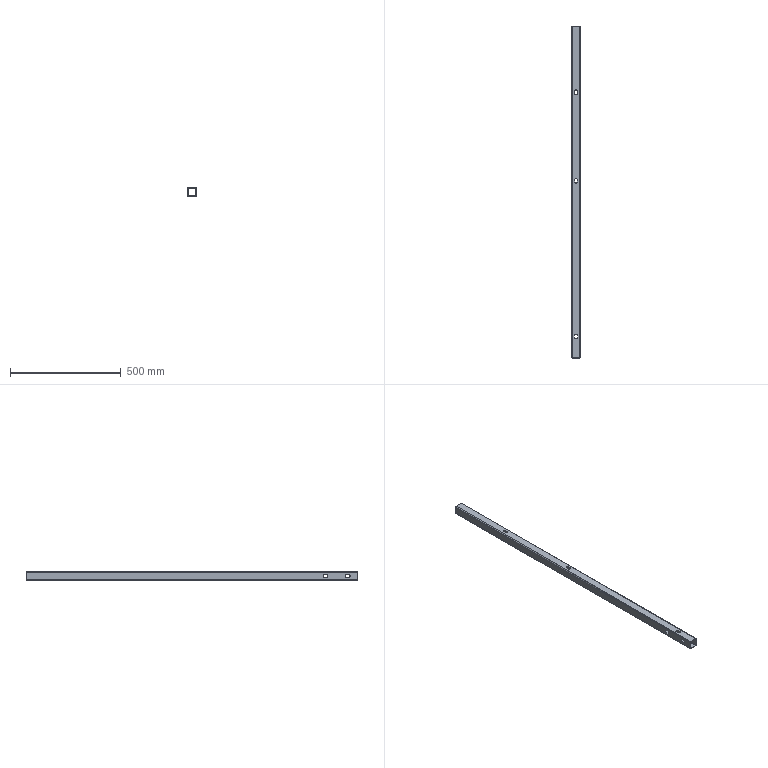Part | STEP file | E3-Powder bin guardrail 8-2 column body_Default<As Machined> | 1 solid | 58 faces | box 40 x 1500 x 40 mm | volume 435692 mm3 | plane 30 | cylinder 28 | commonest cylinder face diameters 12 x16 4 x4 8 x4 15 x4